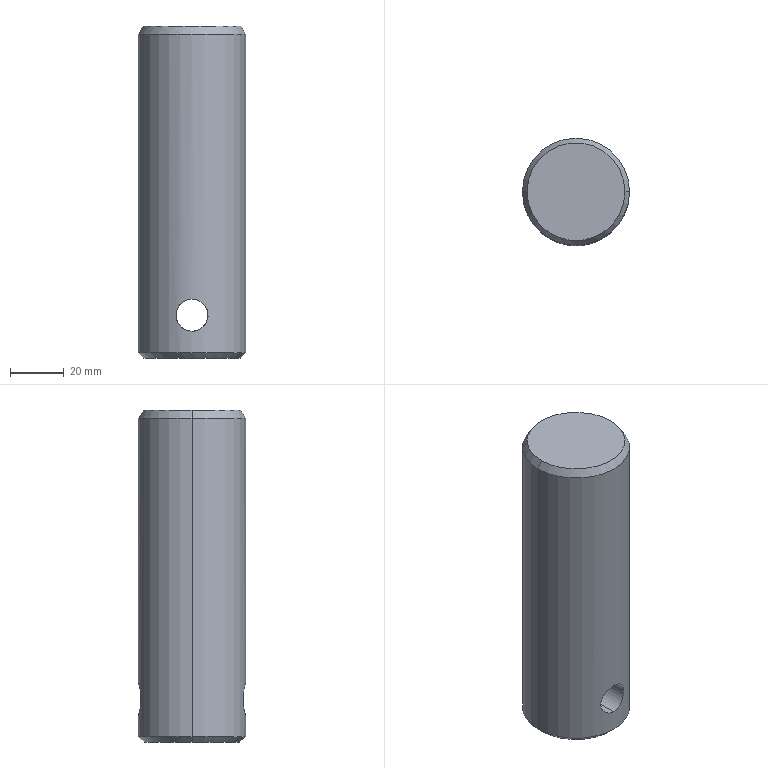Part | SolidWorks | features Chamfer 2, Extrusion 1, ICE 1 | 1 solid | 10 faces | box 40 x 40 x 124 mm | volume 150791 mm3 | cylinder 4 | cone 4 | plane 2 | commonest cylinder face diameters 12 x2 40 x2
STEP:
#1=CARTESIAN_POINT('',(0.,-20.,10.));
#2=VERTEX_POINT('',#1);
#3=CARTESIAN_POINT('',(0.,-20.,22.));
#4=VERTEX_POINT('',#3);
#5=CARTESIAN_POINT('',(0.,-20.,10.));
#6=CARTESIAN_POINT('',(-0.393,-20.,10.));
#7=CARTESIAN_POINT('',(-0.7871,-19.988,10.039));
#8=CARTESIAN_POINT('',(-1.566,-19.942,10.194));
#9=CARTESIAN_POINT('',(-1.941,-19.909,10.309));
#10=CARTESIAN_POINT('',(-2.664,-19.825,10.61));
#11=CARTESIAN_POINT('',(-3.016,-19.774,10.798));
#12=CARTESIAN_POINT('',(-3.665,-19.664,11.233));
#13=CARTESIAN_POINT('',(-3.965,-19.605,11.48));
#14=CARTESIAN_POINT('',(-4.381,-19.515,11.895));
#15=CARTESIAN_POINT('',(-4.513,-19.484,12.042));
#16=CARTESIAN_POINT('',(-4.762,-19.425,12.344));
#17=CARTESIAN_POINT('',(-4.878,-19.396,12.501));
#18=CARTESIAN_POINT('',(-5.202,-19.313,12.986));
#19=CARTESIAN_POINT('',(-5.388,-19.261,13.33));
#20=CARTESIAN_POINT('',(-5.692,-19.174,14.061));
#21=CARTESIAN_POINT('',(-5.806,-19.139,14.436));
#22=CARTESIAN_POINT('',(-5.922,-19.103,15.013));
#23=CARTESIAN_POINT('',(-5.951,-19.094,15.208));
#24=CARTESIAN_POINT('',(-5.99,-19.082,15.602));
#25=CARTESIAN_POINT('',(-6.,-19.079,15.802));
#26=CARTESIAN_POINT('',(-6.,-19.079,16.395));
#27=CARTESIAN_POINT('',(-5.961,-19.091,16.786));
#28=CARTESIAN_POINT('',(-5.846,-19.127,17.366));
#29=CARTESIAN_POINT('',(-5.797,-19.141,17.559));
#30=CARTESIAN_POINT('',(-5.682,-19.176,17.937));
#31=CARTESIAN_POINT('',(-5.616,-19.196,18.122));
#32=CARTESIAN_POINT('',(-5.39,-19.261,18.664));
#33=CARTESIAN_POINT('',(-5.206,-19.312,19.009));
#34=CARTESIAN_POINT('',(-4.767,-19.425,19.665));
#35=CARTESIAN_POINT('',(-4.519,-19.485,19.966));
#36=CARTESIAN_POINT('',(-4.107,-19.574,20.379));
#37=CARTESIAN_POINT('',(-3.963,-19.604,20.51));
#38=CARTESIAN_POINT('',(-3.66,-19.663,20.759));
#39=CARTESIAN_POINT('',(-3.501,-19.692,20.877));
#40=CARTESIAN_POINT('',(-3.013,-19.774,21.203));
#41=CARTESIAN_POINT('',(-2.67,-19.824,21.388));
#42=CARTESIAN_POINT('',(-1.946,-19.908,21.689));
#43=CARTESIAN_POINT('',(-1.563,-19.943,21.806));
#44=CARTESIAN_POINT('',(-0.7911,-19.988,21.961));
#45=CARTESIAN_POINT('',(-0.3988,-20.,22.));
#46=CARTESIAN_POINT('',(0.,-20.,22.));
#47=B_SPLINE_CURVE_WITH_KNOTS('',3,(#5,#6,#7,#8,#9,#10,#11,#12,#13,#14,#15,#16,#17,#18,#19,#20,#21,#22,#23,#24,#25,#26,#27,#28,#29,#30,#31,#32,#33,#34,#35,#36,#37,#38,#39,#40,#41,#42,#43,#44,#45,#46),.UNSPECIFIED.,.F.,.F.,(4,2,2,2,2,2,2,2,2,2,2,2,2,2,2,2,2,2,2,2,4),(0.01887,0.02005,0.02123,0.0224,0.02358,0.02417,0.02476,0.02594,0.02712,0.02771,0.0283,0.02948,0.03007,0.03066,0.03184,0.03302,0.0336,0.03419,0.03537,0.03655,0.03773),.UNSPECIFIED.);
#48=EDGE_CURVE('',#2,#4,#47,.T.);
#49=ORIENTED_EDGE('',*,*,#48,.F.);
#50=CARTESIAN_POINT('',(0.,20.,10.));
#51=VERTEX_POINT('',#50);
#52=CARTESIAN_POINT('',(0.,-20.,10.));
#53=DIRECTION('',(0.,1.,0.));
#54=VECTOR('',#53,1000.);
#55=LINE('',#52,#54);
#56=EDGE_CURVE('',#2,#51,#55,.T.);
#57=ORIENTED_EDGE('',*,*,#56,.T.);
#58=CARTESIAN_POINT('',(0.,20.,22.));
#59=VERTEX_POINT('',#58);
#60=CARTESIAN_POINT('',(0.,20.,22.));
#61=CARTESIAN_POINT('',(-0.3989,20.,22.));
#62=CARTESIAN_POINT('',(-0.7907,19.988,21.961));
#63=CARTESIAN_POINT('',(-1.368,19.954,21.845));
#64=CARTESIAN_POINT('',(-1.559,19.94,21.797));
#65=CARTESIAN_POINT('',(-1.937,19.907,21.682));
#66=CARTESIAN_POINT('',(-2.125,19.888,21.615));
#67=CARTESIAN_POINT('',(-2.669,19.824,21.388));
#68=CARTESIAN_POINT('',(-3.013,19.775,21.204));
#69=CARTESIAN_POINT('',(-3.501,19.692,20.877));
#70=CARTESIAN_POINT('',(-3.659,19.663,20.759));
#71=CARTESIAN_POINT('',(-3.962,19.604,20.51));
#72=CARTESIAN_POINT('',(-4.107,19.574,20.379));
#73=CARTESIAN_POINT('',(-4.519,19.485,19.966));
#74=CARTESIAN_POINT('',(-4.767,19.425,19.665));
#75=CARTESIAN_POINT('',(-5.205,19.312,19.01));
#76=CARTESIAN_POINT('',(-5.39,19.261,18.665));
#77=CARTESIAN_POINT('',(-5.615,19.196,18.124));
#78=CARTESIAN_POINT('',(-5.681,19.176,17.94));
#79=CARTESIAN_POINT('',(-5.796,19.142,17.563));
#80=CARTESIAN_POINT('',(-5.845,19.127,17.369));
#81=CARTESIAN_POINT('',(-5.961,19.091,16.788));
#82=CARTESIAN_POINT('',(-6.,19.079,16.397));
#83=CARTESIAN_POINT('',(-6.,19.079,15.609));
#84=CARTESIAN_POINT('',(-5.961,19.091,15.209));
#85=CARTESIAN_POINT('',(-5.806,19.139,14.437));
#86=CARTESIAN_POINT('',(-5.692,19.174,14.062));
#87=CARTESIAN_POINT('',(-5.389,19.261,13.333));
#88=CARTESIAN_POINT('',(-5.202,19.313,12.985));
#89=CARTESIAN_POINT('',(-4.877,19.397,12.5));
#90=CARTESIAN_POINT('',(-4.761,19.425,12.343));
#91=CARTESIAN_POINT('',(-4.513,19.485,12.041));
#92=CARTESIAN_POINT('',(-4.38,19.515,11.894));
#93=CARTESIAN_POINT('',(-3.964,19.605,11.479));
#94=CARTESIAN_POINT('',(-3.664,19.664,11.232));
#95=CARTESIAN_POINT('',(-3.015,19.774,10.798));
#96=CARTESIAN_POINT('',(-2.664,19.825,10.61));
#97=CARTESIAN_POINT('',(-1.941,19.909,10.309));
#98=CARTESIAN_POINT('',(-1.566,19.942,10.195));
#99=CARTESIAN_POINT('',(-0.985,19.977,10.078));
#100=CARTESIAN_POINT('',(-0.787,19.985,10.049));
#101=CARTESIAN_POINT('',(-0.3932,19.997,10.01));
#102=CARTESIAN_POINT('',(-0.1965,20.,10.));
#103=CARTESIAN_POINT('',(0.,20.,10.));
#104=B_SPLINE_CURVE_WITH_KNOTS('',3,(#60,#61,#62,#63,#64,#65,#66,#67,#68,#69,#70,#71,#72,#73,#74,#75,#76,#77,#78,#79,#80,#81,#82,#83,#84,#85,#86,#87,#88,#89,#90,#91,#92,#93,#94,#95,#96,#97,#98,#99,#100,#101,#102,#103),.UNSPECIFIED.,.F.,.F.,(4,2,2,2,2,2,2,2,2,2,2,2,2,2,2,2,2,2,2,2,2,4),(0.,0.001179,0.001769,0.002359,0.003538,0.004127,0.004717,0.005896,0.007076,0.007665,0.008255,0.009434,0.01061,0.01179,0.01297,0.01356,0.01415,0.01533,0.01651,0.01769,0.01828,0.01887),.UNSPECIFIED.);
#105=EDGE_CURVE('',#59,#51,#104,.T.);
#106=ORIENTED_EDGE('',*,*,#105,.F.);
#107=CARTESIAN_POINT('',(0.,-20.,22.));
#108=DIRECTION('',(0.,1.,0.));
#109=VECTOR('',#108,1000.);
#110=LINE('',#107,#109);
#111=EDGE_CURVE('',#4,#59,#110,.T.);
#112=ORIENTED_EDGE('',*,*,#111,.F.);
#113=EDGE_LOOP('',(#49,#57,#106,#112));
#114=FACE_OUTER_BOUND('',#113,.T.);
#115=CARTESIAN_POINT('',(0.,-20.,16.));
#116=DIRECTION('',(0.,1.,0.));
#117=DIRECTION('',(0.,0.,1.));
#118=AXIS2_PLACEMENT_3D('',#115,#116,#117);
#119=CYLINDRICAL_SURFACE('',#118,6.);
#120=ADVANCED_FACE('',(#114),#119,.F.);
#121=CARTESIAN_POINT('',(-18.,0.,0.));
#122=VERTEX_POINT('',#121);
#123=CARTESIAN_POINT('',(18.,0.,0.));
#124=VERTEX_POINT('',#123);
#125=CARTESIAN_POINT('',(0.,0.,0.));
#126=DIRECTION('',(0.,0.,-1.));
#127=DIRECTION('',(1.,0.,0.));
#128=AXIS2_PLACEMENT_3D('',#125,#126,#127);
#129=CIRCLE('',#128,18.);
#130=EDGE_CURVE('',#122,#124,#129,.T.);
#131=ORIENTED_EDGE('',*,*,#130,.F.);
#132=CARTESIAN_POINT('',(-20.,0.,2.));
#133=VERTEX_POINT('',#132);
#134=CARTESIAN_POINT('',(-20.,0.,2.));
#135=DIRECTION('',(-0.7071,0.,0.7071));
#136=VECTOR('',#135,1000.);
#137=LINE('',#134,#136);
#138=EDGE_CURVE('',#122,#133,#137,.T.);
#139=ORIENTED_EDGE('',*,*,#138,.T.);
#140=CARTESIAN_POINT('',(20.,0.,2.));
#141=VERTEX_POINT('',#140);
#142=CARTESIAN_POINT('',(0.,0.,2.));
#143=DIRECTION('',(0.,0.,1.));
#144=DIRECTION('',(1.,0.,0.));
#145=AXIS2_PLACEMENT_3D('',#142,#143,#144);
#146=CIRCLE('',#145,20.);
#147=EDGE_CURVE('',#141,#133,#146,.T.);
#148=ORIENTED_EDGE('',*,*,#147,.F.);
#149=CARTESIAN_POINT('',(20.,0.,2.));
#150=DIRECTION('',(0.7071,0.,0.7071));
#151=VECTOR('',#150,1000.);
#152=LINE('',#149,#151);
#153=EDGE_CURVE('',#124,#141,#152,.T.);
#154=ORIENTED_EDGE('',*,*,#153,.F.);
#155=EDGE_LOOP('',(#131,#139,#148,#154));
#156=FACE_OUTER_BOUND('',#155,.T.);
#157=CARTESIAN_POINT('',(0.,0.,2.));
#158=DIRECTION('',(0.,0.,1.));
#159=DIRECTION('',(1.,0.,0.));
#160=AXIS2_PLACEMENT_3D('',#157,#158,#159);
#161=CONICAL_SURFACE('',#160,20.,0.7854);
#162=ADVANCED_FACE('',(#156),#161,.T.);
#163=CARTESIAN_POINT('',(18.268,0.,124.));
#164=VERTEX_POINT('',#163);
#165=CARTESIAN_POINT('',(-18.268,0.,124.));
#166=VERTEX_POINT('',#165);
#167=CARTESIAN_POINT('',(0.,0.,124.));
#168=DIRECTION('',(0.,0.,1.));
#169=DIRECTION('',(1.,0.,0.));
#170=AXIS2_PLACEMENT_3D('',#167,#168,#169);
#171=CIRCLE('',#170,18.268);
#172=EDGE_CURVE('',#164,#166,#171,.T.);
#173=ORIENTED_EDGE('',*,*,#172,.F.);
#174=CARTESIAN_POINT('',(20.,0.,121.));
#175=VERTEX_POINT('',#174);
#176=CARTESIAN_POINT('',(18.268,0.,124.));
#177=DIRECTION('',(0.5,0.,-0.866));
#178=VECTOR('',#177,1000.);
#179=LINE('',#176,#178);
#180=EDGE_CURVE('',#164,#175,#179,.T.);
#181=ORIENTED_EDGE('',*,*,#180,.T.);
#182=CARTESIAN_POINT('',(-20.,0.,121.));
#183=VERTEX_POINT('',#182);
#184=CARTESIAN_POINT('',(0.,0.,121.));
#185=DIRECTION('',(0.,0.,-1.));
#186=DIRECTION('',(1.,0.,0.));
#187=AXIS2_PLACEMENT_3D('',#184,#185,#186);
#188=CIRCLE('',#187,20.);
#189=EDGE_CURVE('',#183,#175,#188,.T.);
#190=ORIENTED_EDGE('',*,*,#189,.F.);
#191=CARTESIAN_POINT('',(-18.268,0.,124.));
#192=DIRECTION('',(-0.5,0.,-0.866));
#193=VECTOR('',#192,1000.);
#194=LINE('',#191,#193);
#195=EDGE_CURVE('',#166,#183,#194,.T.);
#196=ORIENTED_EDGE('',*,*,#195,.F.);
#197=EDGE_LOOP('',(#173,#181,#190,#196));
#198=FACE_OUTER_BOUND('',#197,.T.);
#199=CARTESIAN_POINT('',(0.,0.,124.));
#200=DIRECTION('',(0.,0.,-1.));
#201=DIRECTION('',(-1.,0.,0.));
#202=AXIS2_PLACEMENT_3D('',#199,#200,#201);
#203=CONICAL_SURFACE('',#202,18.268,0.5236);
#204=ADVANCED_FACE('',(#198),#203,.T.);
#205=ORIENTED_EDGE('',*,*,#105,.T.);
#206=CARTESIAN_POINT('',(0.,20.,10.));
#207=CARTESIAN_POINT('',(0.393,20.,10.));
#208=CARTESIAN_POINT('',(0.7871,19.988,10.039));
#209=CARTESIAN_POINT('',(1.566,19.942,10.194));
#210=CARTESIAN_POINT('',(1.941,19.909,10.309));
#211=CARTESIAN_POINT('',(2.664,19.825,10.61));
#212=CARTESIAN_POINT('',(3.016,19.774,10.798));
#213=CARTESIAN_POINT('',(3.665,19.664,11.233));
#214=CARTESIAN_POINT('',(3.965,19.605,11.48));
#215=CARTESIAN_POINT('',(4.381,19.515,11.895));
#216=CARTESIAN_POINT('',(4.513,19.484,12.042));
#217=CARTESIAN_POINT('',(4.762,19.425,12.344));
#218=CARTESIAN_POINT('',(4.878,19.396,12.501));
#219=CARTESIAN_POINT('',(5.202,19.313,12.986));
#220=CARTESIAN_POINT('',(5.388,19.261,13.33));
#221=CARTESIAN_POINT('',(5.692,19.174,14.061));
#222=CARTESIAN_POINT('',(5.806,19.139,14.436));
#223=CARTESIAN_POINT('',(5.922,19.103,15.013));
#224=CARTESIAN_POINT('',(5.951,19.094,15.208));
#225=CARTESIAN_POINT('',(5.99,19.082,15.602));
#226=CARTESIAN_POINT('',(6.,19.079,15.802));
#227=CARTESIAN_POINT('',(6.,19.079,16.395));
#228=CARTESIAN_POINT('',(5.961,19.091,16.786));
#229=CARTESIAN_POINT('',(5.846,19.127,17.366));
#230=CARTESIAN_POINT('',(5.797,19.141,17.559));
#231=CARTESIAN_POINT('',(5.682,19.176,17.937));
#232=CARTESIAN_POINT('',(5.616,19.196,18.122));
#233=CARTESIAN_POINT('',(5.39,19.261,18.664));
#234=CARTESIAN_POINT('',(5.206,19.312,19.009));
#235=CARTESIAN_POINT('',(4.767,19.425,19.665));
#236=CARTESIAN_POINT('',(4.519,19.485,19.966));
#237=CARTESIAN_POINT('',(4.107,19.574,20.379));
#238=CARTESIAN_POINT('',(3.963,19.604,20.51));
#239=CARTESIAN_POINT('',(3.66,19.663,20.759));
#240=CARTESIAN_POINT('',(3.501,19.692,20.877));
#241=CARTESIAN_POINT('',(3.013,19.774,21.203));
#242=CARTESIAN_POINT('',(2.67,19.824,21.388));
#243=CARTESIAN_POINT('',(1.946,19.908,21.689));
#244=CARTESIAN_POINT('',(1.563,19.943,21.806));
#245=CARTESIAN_POINT('',(0.7911,19.988,21.961));
#246=CARTESIAN_POINT('',(0.3988,20.,22.));
#247=CARTESIAN_POINT('',(0.,20.,22.));
#248=B_SPLINE_CURVE_WITH_KNOTS('',3,(#206,#207,#208,#209,#210,#211,#212,#213,#214,#215,#216,#217,#218,#219,#220,#221,#222,#223,#224,#225,#226,#227,#228,#229,#230,#231,#232,#233,#234,#235,#236,#237,#238,#239,#240,#241,#242,#243,#244,#245,#246,#247),.UNSPECIFIED.,.F.,.F.,(4,2,2,2,2,2,2,2,2,2,2,2,2,2,2,2,2,2,2,2,4),(0.01887,0.02005,0.02123,0.0224,0.02358,0.02417,0.02476,0.02594,0.02712,0.02771,0.0283,0.02948,0.03007,0.03066,0.03184,0.03302,0.0336,0.03419,0.03537,0.03655,0.03773),.UNSPECIFIED.);
#249=EDGE_CURVE('',#51,#59,#248,.T.);
#250=ORIENTED_EDGE('',*,*,#249,.T.);
#251=EDGE_LOOP('',(#205,#250));
#252=FACE_BOUND('',#251,.T.);
#253=ORIENTED_EDGE('',*,*,#189,.T.);
#254=CARTESIAN_POINT('',(20.,0.,124.));
#255=DIRECTION('',(0.,0.,-1.));
#256=VECTOR('',#255,1000.);
#257=LINE('',#254,#256);
#258=EDGE_CURVE('',#175,#141,#257,.T.);
#259=ORIENTED_EDGE('',*,*,#258,.T.);
#260=ORIENTED_EDGE('',*,*,#147,.T.);
#261=CARTESIAN_POINT('',(-20.,0.,124.));
#262=DIRECTION('',(0.,0.,-1.));
#263=VECTOR('',#262,1000.);
#264=LINE('',#261,#263);
#265=EDGE_CURVE('',#183,#133,#264,.T.);
#266=ORIENTED_EDGE('',*,*,#265,.F.);
#267=EDGE_LOOP('',(#253,#259,#260,#266));
#268=FACE_OUTER_BOUND('',#267,.T.);
#269=CARTESIAN_POINT('',(0.,0.,124.));
#270=DIRECTION('',(0.,0.,-1.));
#271=DIRECTION('',(-1.,0.,0.));
#272=AXIS2_PLACEMENT_3D('',#269,#270,#271);
#273=CYLINDRICAL_SURFACE('',#272,20.);
#274=ADVANCED_FACE('',(#252,#268),#273,.T.);
#275=ORIENTED_EDGE('',*,*,#258,.F.);
#276=CARTESIAN_POINT('',(0.,0.,121.));
#277=DIRECTION('',(0.,0.,-1.));
#278=DIRECTION('',(1.,0.,0.));
#279=AXIS2_PLACEMENT_3D('',#276,#277,#278);
#280=CIRCLE('',#279,20.);
#281=EDGE_CURVE('',#175,#183,#280,.T.);
#282=ORIENTED_EDGE('',*,*,#281,.T.);
#283=ORIENTED_EDGE('',*,*,#265,.T.);
#284=CARTESIAN_POINT('',(0.,0.,2.));
#285=DIRECTION('',(0.,0.,1.));
#286=DIRECTION('',(1.,0.,0.));
#287=AXIS2_PLACEMENT_3D('',#284,#285,#286);
#288=CIRCLE('',#287,20.);
#289=EDGE_CURVE('',#133,#141,#288,.T.);
#290=ORIENTED_EDGE('',*,*,#289,.T.);
#291=EDGE_LOOP('',(#275,#282,#283,#290));
#292=FACE_OUTER_BOUND('',#291,.T.);
#293=CARTESIAN_POINT('',(0.,-20.,22.));
#294=CARTESIAN_POINT('',(0.3989,-20.,22.));
#295=CARTESIAN_POINT('',(0.7907,-19.988,21.961));
#296=CARTESIAN_POINT('',(1.368,-19.954,21.845));
#297=CARTESIAN_POINT('',(1.559,-19.94,21.797));
#298=CARTESIAN_POINT('',(1.937,-19.907,21.682));
#299=CARTESIAN_POINT('',(2.125,-19.888,21.615));
#300=CARTESIAN_POINT('',(2.669,-19.824,21.388));
#301=CARTESIAN_POINT('',(3.013,-19.775,21.204));
#302=CARTESIAN_POINT('',(3.501,-19.692,20.877));
#303=CARTESIAN_POINT('',(3.659,-19.663,20.759));
#304=CARTESIAN_POINT('',(3.962,-19.604,20.51));
#305=CARTESIAN_POINT('',(4.107,-19.574,20.379));
#306=CARTESIAN_POINT('',(4.519,-19.485,19.966));
#307=CARTESIAN_POINT('',(4.767,-19.425,19.665));
#308=CARTESIAN_POINT('',(5.205,-19.312,19.01));
#309=CARTESIAN_POINT('',(5.39,-19.261,18.665));
#310=CARTESIAN_POINT('',(5.615,-19.196,18.124));
#311=CARTESIAN_POINT('',(5.681,-19.176,17.94));
#312=CARTESIAN_POINT('',(5.796,-19.142,17.563));
#313=CARTESIAN_POINT('',(5.845,-19.127,17.369));
#314=CARTESIAN_POINT('',(5.961,-19.091,16.788));
#315=CARTESIAN_POINT('',(6.,-19.079,16.397));
#316=CARTESIAN_POINT('',(6.,-19.079,15.609));
#317=CARTESIAN_POINT('',(5.961,-19.091,15.209));
#318=CARTESIAN_POINT('',(5.806,-19.139,14.437));
#319=CARTESIAN_POINT('',(5.692,-19.174,14.062));
#320=CARTESIAN_POINT('',(5.389,-19.261,13.333));
#321=CARTESIAN_POINT('',(5.202,-19.313,12.985));
#322=CARTESIAN_POINT('',(4.877,-19.397,12.5));
#323=CARTESIAN_POINT('',(4.761,-19.425,12.343));
#324=CARTESIAN_POINT('',(4.513,-19.485,12.041));
#325=CARTESIAN_POINT('',(4.38,-19.515,11.894));
#326=CARTESIAN_POINT('',(3.964,-19.605,11.479));
#327=CARTESIAN_POINT('',(3.664,-19.664,11.232));
#328=CARTESIAN_POINT('',(3.015,-19.774,10.798));
#329=CARTESIAN_POINT('',(2.664,-19.825,10.61));
#330=CARTESIAN_POINT('',(1.941,-19.909,10.309));
#331=CARTESIAN_POINT('',(1.566,-19.942,10.195));
#332=CARTESIAN_POINT('',(0.985,-19.977,10.078));
#333=CARTESIAN_POINT('',(0.787,-19.985,10.049));
#334=CARTESIAN_POINT('',(0.3932,-19.997,10.01));
#335=CARTESIAN_POINT('',(0.1965,-20.,10.));
#336=CARTESIAN_POINT('',(0.,-20.,10.));
#337=B_SPLINE_CURVE_WITH_KNOTS('',3,(#293,#294,#295,#296,#297,#298,#299,#300,#301,#302,#303,#304,#305,#306,#307,#308,#309,#310,#311,#312,#313,#314,#315,#316,#317,#318,#319,#320,#321,#322,#323,#324,#325,#326,#327,#328,#329,#330,#331,#332,#333,#334,#335,#336),.UNSPECIFIED.,.F.,.F.,(4,2,2,2,2,2,2,2,2,2,2,2,2,2,2,2,2,2,2,2,2,4),(0.,0.001179,0.001769,0.002359,0.003538,0.004127,0.004717,0.005896,0.007076,0.007665,0.008255,0.009434,0.01061,0.01179,0.01297,0.01356,0.01415,0.01533,0.01651,0.01769,0.01828,0.01887),.UNSPECIFIED.);
#338=EDGE_CURVE('',#4,#2,#337,.T.);
#339=ORIENTED_EDGE('',*,*,#338,.T.);
#340=ORIENTED_EDGE('',*,*,#48,.T.);
#341=EDGE_LOOP('',(#339,#340));
#342=FACE_BOUND('',#341,.T.);
#343=CARTESIAN_POINT('',(0.,0.,124.));
#344=DIRECTION('',(0.,0.,-1.));
#345=DIRECTION('',(-1.,0.,0.));
#346=AXIS2_PLACEMENT_3D('',#343,#344,#345);
#347=CYLINDRICAL_SURFACE('',#346,20.);
#348=ADVANCED_FACE('',(#292,#342),#347,.T.);
#349=CARTESIAN_POINT('',(0.,0.,124.));
#350=DIRECTION('',(0.,0.,1.));
#351=DIRECTION('',(1.,0.,0.));
#352=AXIS2_PLACEMENT_3D('',#349,#350,#351);
#353=CIRCLE('',#352,18.268);
#354=EDGE_CURVE('',#166,#164,#353,.T.);
#355=ORIENTED_EDGE('',*,*,#354,.T.);
#356=ORIENTED_EDGE('',*,*,#172,.T.);
#357=EDGE_LOOP('',(#355,#356));
#358=FACE_OUTER_BOUND('',#357,.T.);
#359=CARTESIAN_POINT('',(0.,0.,124.));
#360=DIRECTION('',(0.,0.,1.));
#361=DIRECTION('',(1.,0.,0.));
#362=AXIS2_PLACEMENT_3D('',#359,#360,#361);
#363=PLANE('',#362);
#364=ADVANCED_FACE('',(#358),#363,.T.);
#365=CARTESIAN_POINT('',(0.,0.,0.));
#366=DIRECTION('',(0.,0.,-1.));
#367=DIRECTION('',(1.,0.,0.));
#368=AXIS2_PLACEMENT_3D('',#365,#366,#367);
#369=CIRCLE('',#368,18.);
#370=EDGE_CURVE('',#124,#122,#369,.T.);
#371=ORIENTED_EDGE('',*,*,#370,.T.);
#372=ORIENTED_EDGE('',*,*,#130,.T.);
#373=EDGE_LOOP('',(#371,#372));
#374=FACE_OUTER_BOUND('',#373,.T.);
#375=CARTESIAN_POINT('',(0.,0.,0.));
#376=DIRECTION('',(0.,0.,1.));
#377=DIRECTION('',(1.,0.,0.));
#378=AXIS2_PLACEMENT_3D('',#375,#376,#377);
#379=PLANE('',#378);
#380=ADVANCED_FACE('',(#374),#379,.F.);
#381=ORIENTED_EDGE('',*,*,#180,.F.);
#382=ORIENTED_EDGE('',*,*,#354,.F.);
#383=ORIENTED_EDGE('',*,*,#195,.T.);
#384=ORIENTED_EDGE('',*,*,#281,.F.);
#385=EDGE_LOOP('',(#381,#382,#383,#384));
#386=FACE_OUTER_BOUND('',#385,.T.);
#387=CARTESIAN_POINT('',(0.,0.,124.));
#388=DIRECTION('',(0.,0.,-1.));
#389=DIRECTION('',(-1.,0.,0.));
#390=AXIS2_PLACEMENT_3D('',#387,#388,#389);
#391=CONICAL_SURFACE('',#390,18.268,0.5236);
#392=ADVANCED_FACE('',(#386),#391,.T.);
#393=ORIENTED_EDGE('',*,*,#138,.F.);
#394=ORIENTED_EDGE('',*,*,#370,.F.);
#395=ORIENTED_EDGE('',*,*,#153,.T.);
#396=ORIENTED_EDGE('',*,*,#289,.F.);
#397=EDGE_LOOP('',(#393,#394,#395,#396));
#398=FACE_OUTER_BOUND('',#397,.T.);
#399=CARTESIAN_POINT('',(0.,0.,2.));
#400=DIRECTION('',(0.,0.,1.));
#401=DIRECTION('',(1.,0.,0.));
#402=AXIS2_PLACEMENT_3D('',#399,#400,#401);
#403=CONICAL_SURFACE('',#402,20.,0.7854);
#404=ADVANCED_FACE('',(#398),#403,.T.);
#405=ORIENTED_EDGE('',*,*,#56,.F.);
#406=ORIENTED_EDGE('',*,*,#338,.F.);
#407=ORIENTED_EDGE('',*,*,#111,.T.);
#408=ORIENTED_EDGE('',*,*,#249,.F.);
#409=EDGE_LOOP('',(#405,#406,#407,#408));
#410=FACE_OUTER_BOUND('',#409,.T.);
#411=CARTESIAN_POINT('',(0.,-20.,16.));
#412=DIRECTION('',(0.,1.,0.));
#413=DIRECTION('',(0.,0.,1.));
#414=AXIS2_PLACEMENT_3D('',#411,#412,#413);
#415=CYLINDRICAL_SURFACE('',#414,6.);
#416=ADVANCED_FACE('',(#410),#415,.F.);
#417=CLOSED_SHELL('',(#120,#162,#204,#274,#348,#364,#380,#392,#404,#416));
#418=MANIFOLD_SOLID_BREP('',#417);
#419=CARTESIAN_POINT('',(0.,0.,0.));
#420=DIRECTION('',(0.,0.,1.));
#421=DIRECTION('',(1.,0.,0.));
#422=AXIS2_PLACEMENT_3D('',#419,#420,#421);
#423=(LENGTH_UNIT()NAMED_UNIT(*)SI_UNIT(.MILLI.,.METRE.));
#424=UNCERTAINTY_MEASURE_WITH_UNIT(LENGTH_MEASURE(0.00001),#423,'','');
#425=(NAMED_UNIT(*)PLANE_ANGLE_UNIT()SI_UNIT($,.RADIAN.));
#426=(NAMED_UNIT(*)SI_UNIT($,.STERADIAN.)SOLID_ANGLE_UNIT());
#427=(GEOMETRIC_REPRESENTATION_CONTEXT(3)GLOBAL_UNCERTAINTY_ASSIGNED_CONTEXT((#424))GLOBAL_UNIT_ASSIGNED_CONTEXT((#423,#425,#426))REPRESENTATION_CONTEXT('',''));
#428=ADVANCED_BREP_SHAPE_REPRESENTATION('',(#418,#422),#427);